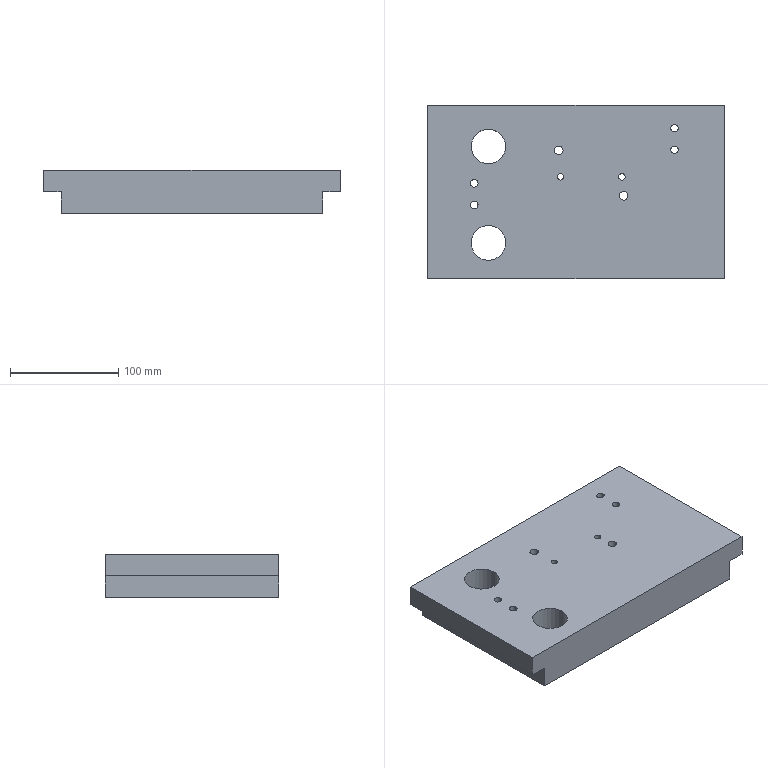Part | 1 solid | 67 faces | box 273.935 x 160 x 40 mm | volume 1409824 mm3 | cylinder 36 | plane 19 | cone 12 | commonest cylinder face diameters 8 x12 7 x8 6 x4 10 x4 32 x4 34 x4